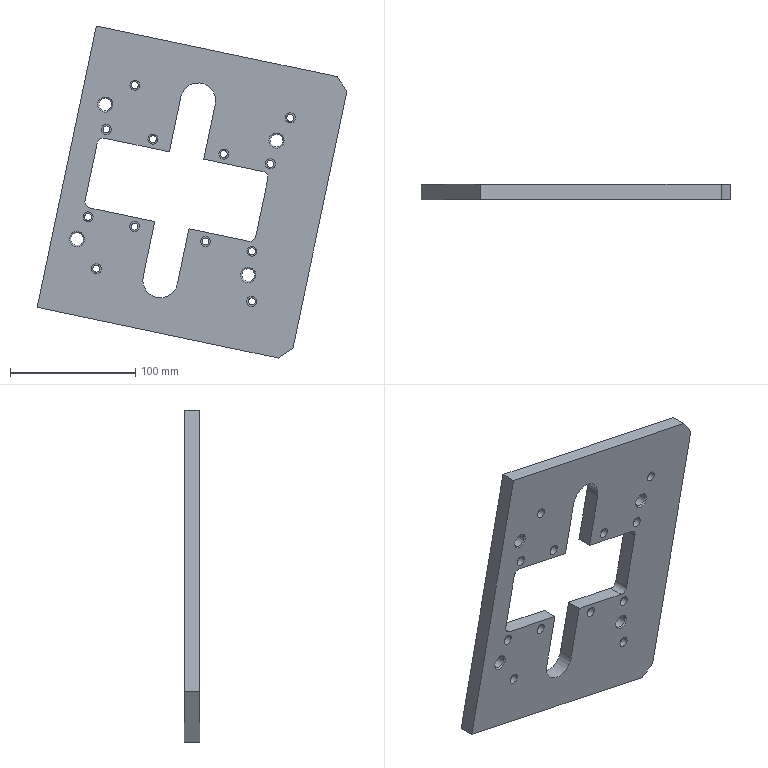Part | STEP file | BERCO_002 | 1 solid | 68 faces | box 247.817 x 12 x 265.596 mm | volume 428406 mm3 | cylinder 34 | plane 30 | cone 4 | commonest cylinder face diameters 5.5 x12 8 x12 10 x4 10.1 x4 28 x2